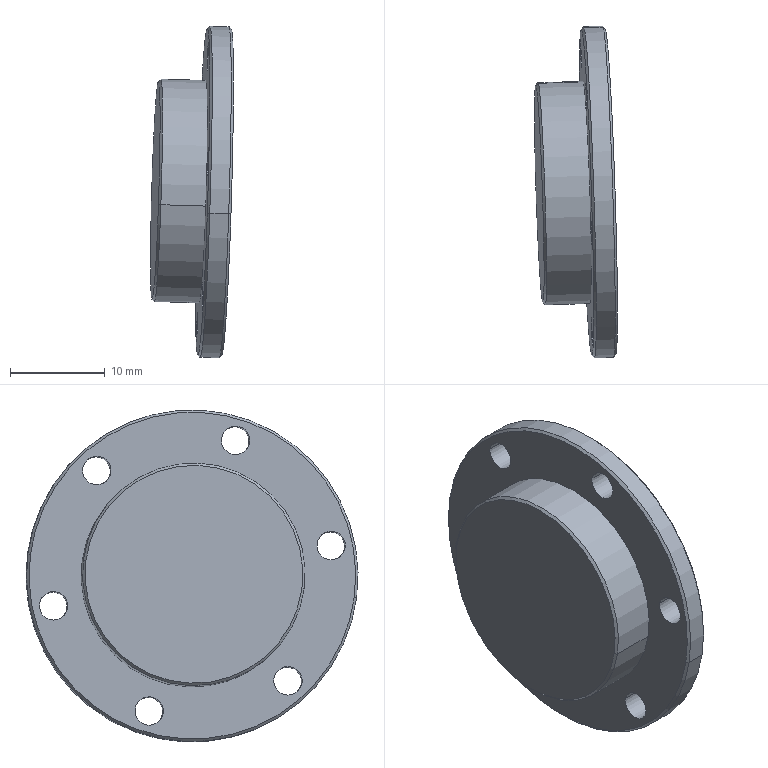Part | STEP file | 2026.6.15-Main Assembly图.sldasm-Part-114 | 1 solid | 30 faces | box 8.754 x 35.047 x 35.043 mm | volume 2415 mm3 | cylinder 18 | cone 8 | plane 4 | commonest cylinder face diameters 3 x12 20 x2 23.5 x2 35 x2
STEP:
#1=CARTESIAN_POINT('',(-1578.328,1431.126,3695.117));
#2=VERTEX_POINT('',#1);
#3=CARTESIAN_POINT('',(-1577.667,1408.329,3692.14));
#4=VERTEX_POINT('',#3);
#5=CARTESIAN_POINT('',(-1577.997,1419.728,3693.629));
#6=DIRECTION('',(-0.999,-0.03277,0.02917));
#7=DIRECTION('',(-0.02873,0.9912,0.1295));
#8=AXIS2_PLACEMENT_3D('',#5,#6,#7);
#9=CIRCLE('',#8,11.5);
#10=EDGE_CURVE('',#2,#4,#9,.T.);
#11=ORIENTED_EDGE('',*,*,#10,.F.);
#12=CARTESIAN_POINT('',(-1578.085,1431.382,3695.143));
#13=VERTEX_POINT('',#12);
#14=CARTESIAN_POINT('',(-1578.328,1431.126,3695.117));
#15=DIRECTION('',(0.6861,0.724,0.07092));
#16=VECTOR('',#15,1000.);
#17=LINE('',#14,#16);
#18=EDGE_CURVE('',#2,#13,#17,.T.);
#19=ORIENTED_EDGE('',*,*,#18,.T.);
#20=CARTESIAN_POINT('',(-1577.41,1408.09,3692.1));
#21=VERTEX_POINT('',#20);
#22=CARTESIAN_POINT('',(-1577.747,1419.736,3693.621));
#23=DIRECTION('',(0.999,0.03277,-0.02917));
#24=DIRECTION('',(-0.02873,0.9912,0.1295));
#25=AXIS2_PLACEMENT_3D('',#22,#23,#24);
#26=CIRCLE('',#25,11.75);
#27=EDGE_CURVE('',#21,#13,#26,.T.);
#28=ORIENTED_EDGE('',*,*,#27,.F.);
#29=CARTESIAN_POINT('',(-1577.667,1408.329,3692.14));
#30=DIRECTION('',(0.7267,-0.6777,-0.1122));
#31=VECTOR('',#30,1000.);
#32=LINE('',#29,#31);
#33=EDGE_CURVE('',#4,#21,#32,.T.);
#34=ORIENTED_EDGE('',*,*,#33,.F.);
#35=EDGE_LOOP('',(#11,#19,#28,#34));
#36=FACE_OUTER_BOUND('',#35,.T.);
#37=CARTESIAN_POINT('',(-1577.997,1419.728,3693.629));
#38=DIRECTION('',(0.999,0.03277,-0.02917));
#39=DIRECTION('',(0.02873,-0.9912,-0.1295));
#40=AXIS2_PLACEMENT_3D('',#37,#38,#39);
#41=CONICAL_SURFACE('',#40,11.5,0.7854);
#42=ADVANCED_FACE('',(#36),#41,.T.);
#43=CARTESIAN_POINT('',(-1573.498,1436.989,3695.716));
#44=VERTEX_POINT('',#43);
#45=CARTESIAN_POINT('',(-1572.506,1402.794,3691.249));
#46=VERTEX_POINT('',#45);
#47=CARTESIAN_POINT('',(-1573.002,1419.891,3693.483));
#48=DIRECTION('',(-0.999,-0.03277,0.02917));
#49=DIRECTION('',(-0.02873,0.9912,0.1295));
#50=AXIS2_PLACEMENT_3D('',#47,#48,#49);
#51=CIRCLE('',#50,17.25);
#52=EDGE_CURVE('',#44,#46,#51,.T.);
#53=ORIENTED_EDGE('',*,*,#52,.F.);
#54=CARTESIAN_POINT('',(-1573.255,1437.245,3695.741));
#55=VERTEX_POINT('',#54);
#56=CARTESIAN_POINT('',(-1573.498,1436.989,3695.716));
#57=DIRECTION('',(0.6861,0.724,0.07092));
#58=VECTOR('',#57,1000.);
#59=LINE('',#56,#58);
#60=EDGE_CURVE('',#44,#55,#59,.T.);
#61=ORIENTED_EDGE('',*,*,#60,.T.);
#62=CARTESIAN_POINT('',(-1572.249,1402.554,3691.21));
#63=VERTEX_POINT('',#62);
#64=CARTESIAN_POINT('',(-1572.752,1419.9,3693.475));
#65=DIRECTION('',(0.999,0.03277,-0.02917));
#66=DIRECTION('',(-0.02873,0.9912,0.1295));
#67=AXIS2_PLACEMENT_3D('',#64,#65,#66);
#68=CIRCLE('',#67,17.5);
#69=EDGE_CURVE('',#63,#55,#68,.T.);
#70=ORIENTED_EDGE('',*,*,#69,.F.);
#71=CARTESIAN_POINT('',(-1572.506,1402.794,3691.249));
#72=DIRECTION('',(0.7267,-0.6777,-0.1122));
#73=VECTOR('',#72,1000.);
#74=LINE('',#71,#73);
#75=EDGE_CURVE('',#46,#63,#74,.T.);
#76=ORIENTED_EDGE('',*,*,#75,.F.);
#77=EDGE_LOOP('',(#53,#61,#70,#76));
#78=FACE_OUTER_BOUND('',#77,.T.);
#79=CARTESIAN_POINT('',(-1573.002,1419.891,3693.483));
#80=DIRECTION('',(0.999,0.03277,-0.02917));
#81=DIRECTION('',(0.02873,-0.9912,-0.1295));
#82=AXIS2_PLACEMENT_3D('',#79,#80,#81);
#83=CONICAL_SURFACE('',#82,17.25,0.7854);
#84=ADVANCED_FACE('',(#78),#83,.T.);
#85=CARTESIAN_POINT('',(-1570.009,1402.876,3691.176));
#86=VERTEX_POINT('',#85);
#87=CARTESIAN_POINT('',(-1571.,1437.071,3695.643));
#88=VERTEX_POINT('',#87);
#89=CARTESIAN_POINT('',(-1570.504,1419.973,3693.41));
#90=DIRECTION('',(0.999,0.03277,-0.02917));
#91=DIRECTION('',(-0.02873,0.9912,0.1295));
#92=AXIS2_PLACEMENT_3D('',#89,#90,#91);
#93=CIRCLE('',#92,17.25);
#94=EDGE_CURVE('',#86,#88,#93,.T.);
#95=ORIENTED_EDGE('',*,*,#94,.F.);
#96=CARTESIAN_POINT('',(-1570.251,1402.62,3691.151));
#97=VERTEX_POINT('',#96);
#98=CARTESIAN_POINT('',(-1570.251,1402.62,3691.151));
#99=DIRECTION('',(-0.6861,-0.724,-0.07092));
#100=VECTOR('',#99,1000.);
#101=LINE('',#98,#100);
#102=EDGE_CURVE('',#86,#97,#101,.T.);
#103=ORIENTED_EDGE('',*,*,#102,.T.);
#104=CARTESIAN_POINT('',(-1571.257,1437.311,3695.683));
#105=VERTEX_POINT('',#104);
#106=CARTESIAN_POINT('',(-1570.754,1419.965,3693.417));
#107=DIRECTION('',(-0.999,-0.03277,0.02917));
#108=DIRECTION('',(-0.02873,0.9912,0.1295));
#109=AXIS2_PLACEMENT_3D('',#106,#107,#108);
#110=CIRCLE('',#109,17.5);
#111=EDGE_CURVE('',#105,#97,#110,.T.);
#112=ORIENTED_EDGE('',*,*,#111,.F.);
#113=CARTESIAN_POINT('',(-1571.257,1437.311,3695.683));
#114=DIRECTION('',(-0.7267,0.6777,0.1122));
#115=VECTOR('',#114,1000.);
#116=LINE('',#113,#115);
#117=EDGE_CURVE('',#88,#105,#116,.T.);
#118=ORIENTED_EDGE('',*,*,#117,.F.);
#119=EDGE_LOOP('',(#95,#103,#112,#118));
#120=FACE_OUTER_BOUND('',#119,.T.);
#121=CARTESIAN_POINT('',(-1570.754,1419.965,3693.417));
#122=DIRECTION('',(-0.999,-0.03277,0.02917));
#123=DIRECTION('',(-0.02873,0.9912,0.1295));
#124=AXIS2_PLACEMENT_3D('',#121,#122,#123);
#125=CONICAL_SURFACE('',#124,17.5,0.7854);
#126=ADVANCED_FACE('',(#120),#125,.T.);
#127=CARTESIAN_POINT('',(-1571.041,1429.877,3694.712));
#128=VERTEX_POINT('',#127);
#129=CARTESIAN_POINT('',(-1570.467,1410.053,3692.122));
#130=VERTEX_POINT('',#129);
#131=CARTESIAN_POINT('',(-1570.754,1419.965,3693.417));
#132=DIRECTION('',(0.999,0.03277,-0.02917));
#133=DIRECTION('',(-0.02873,0.9912,0.1295));
#134=AXIS2_PLACEMENT_3D('',#131,#132,#133);
#135=CIRCLE('',#134,10.);
#136=EDGE_CURVE('',#128,#130,#135,.T.);
#137=ORIENTED_EDGE('',*,*,#136,.F.);
#138=CARTESIAN_POINT('',(-1570.799,1430.133,3694.737));
#139=VERTEX_POINT('',#138);
#140=CARTESIAN_POINT('',(-1570.799,1430.133,3694.737));
#141=DIRECTION('',(0.6861,0.724,0.07092));
#142=VECTOR('',#141,1000.);
#143=LINE('',#140,#142);
#144=EDGE_CURVE('',#128,#139,#143,.T.);
#145=ORIENTED_EDGE('',*,*,#144,.T.);
#146=CARTESIAN_POINT('',(-1570.21,1409.814,3692.083));
#147=VERTEX_POINT('',#146);
#148=CARTESIAN_POINT('',(-1570.504,1419.973,3693.41));
#149=DIRECTION('',(-0.999,-0.03277,0.02917));
#150=DIRECTION('',(-0.02873,0.9912,0.1295));
#151=AXIS2_PLACEMENT_3D('',#148,#149,#150);
#152=CIRCLE('',#151,10.25);
#153=EDGE_CURVE('',#147,#139,#152,.T.);
#154=ORIENTED_EDGE('',*,*,#153,.F.);
#155=CARTESIAN_POINT('',(-1570.21,1409.814,3692.083));
#156=DIRECTION('',(0.7267,-0.6777,-0.1122));
#157=VECTOR('',#156,1000.);
#158=LINE('',#155,#157);
#159=EDGE_CURVE('',#130,#147,#158,.T.);
#160=ORIENTED_EDGE('',*,*,#159,.F.);
#161=EDGE_LOOP('',(#137,#145,#154,#160));
#162=FACE_OUTER_BOUND('',#161,.T.);
#163=CARTESIAN_POINT('',(-1570.504,1419.973,3693.41));
#164=DIRECTION('',(0.999,0.03277,-0.02917));
#165=DIRECTION('',(0.02873,-0.9912,-0.1295));
#166=AXIS2_PLACEMENT_3D('',#163,#164,#165);
#167=CONICAL_SURFACE('',#166,10.25,0.7854);
#168=ADVANCED_FACE('',(#162),#167,.F.);
#169=ORIENTED_EDGE('',*,*,#136,.T.);
#170=CARTESIAN_POINT('',(-1576.711,1409.849,3692.305));
#171=VERTEX_POINT('',#170);
#172=CARTESIAN_POINT('',(-1569.718,1410.078,3692.1));
#173=DIRECTION('',(-0.999,-0.03277,0.02917));
#174=VECTOR('',#173,1000.);
#175=LINE('',#172,#174);
#176=EDGE_CURVE('',#130,#171,#175,.T.);
#177=ORIENTED_EDGE('',*,*,#176,.T.);
#178=CARTESIAN_POINT('',(-1577.285,1429.672,3694.894));
#179=VERTEX_POINT('',#178);
#180=CARTESIAN_POINT('',(-1576.998,1419.76,3693.599));
#181=DIRECTION('',(0.999,0.03277,-0.02917));
#182=DIRECTION('',(-0.04387,0.7391,-0.6721));
#183=AXIS2_PLACEMENT_3D('',#180,#181,#182);
#184=CIRCLE('',#183,10.);
#185=EDGE_CURVE('',#179,#171,#184,.T.);
#186=ORIENTED_EDGE('',*,*,#185,.F.);
#187=CARTESIAN_POINT('',(-1570.292,1429.901,3694.69));
#188=DIRECTION('',(-0.999,-0.03277,0.02917));
#189=VECTOR('',#188,1000.);
#190=LINE('',#187,#189);
#191=EDGE_CURVE('',#128,#179,#190,.T.);
#192=ORIENTED_EDGE('',*,*,#191,.F.);
#193=EDGE_LOOP('',(#169,#177,#186,#192));
#194=FACE_OUTER_BOUND('',#193,.T.);
#195=CARTESIAN_POINT('',(-1570.005,1419.99,3693.395));
#196=DIRECTION('',(-0.999,-0.03277,0.02917));
#197=DIRECTION('',(-0.02873,0.9912,0.1295));
#198=AXIS2_PLACEMENT_3D('',#195,#196,#197);
#199=CYLINDRICAL_SURFACE('',#198,10.);
#200=ADVANCED_FACE('',(#194),#199,.F.);
#201=CARTESIAN_POINT('',(-1571.035,1433.134,3690.033));
#202=VERTEX_POINT('',#201);
#203=CARTESIAN_POINT('',(-1571.121,1436.107,3690.422));
#204=VERTEX_POINT('',#203);
#205=CARTESIAN_POINT('',(-1571.078,1434.621,3690.227));
#206=DIRECTION('',(-0.999,-0.03277,0.02917));
#207=DIRECTION('',(-0.04387,0.7391,-0.6721));
#208=AXIS2_PLACEMENT_3D('',#205,#206,#207);
#209=CIRCLE('',#208,1.5);
#210=EDGE_CURVE('',#202,#204,#209,.T.);
#211=ORIENTED_EDGE('',*,*,#210,.F.);
#212=CARTESIAN_POINT('',(-1573.532,1433.052,3690.106));
#213=VERTEX_POINT('',#212);
#214=CARTESIAN_POINT('',(-1571.035,1433.134,3690.033));
#215=DIRECTION('',(-0.999,-0.03277,0.02917));
#216=VECTOR('',#215,1000.);
#217=LINE('',#214,#216);
#218=EDGE_CURVE('',#202,#213,#217,.T.);
#219=ORIENTED_EDGE('',*,*,#218,.T.);
#220=CARTESIAN_POINT('',(-1573.618,1436.025,3690.495));
#221=VERTEX_POINT('',#220);
#222=CARTESIAN_POINT('',(-1573.575,1434.539,3690.3));
#223=DIRECTION('',(-0.999,-0.03277,0.02917));
#224=DIRECTION('',(-0.04387,0.7391,-0.6721));
#225=AXIS2_PLACEMENT_3D('',#222,#223,#224);
#226=CIRCLE('',#225,1.5);
#227=EDGE_CURVE('',#213,#221,#226,.T.);
#228=ORIENTED_EDGE('',*,*,#227,.T.);
#229=CARTESIAN_POINT('',(-1571.121,1436.107,3690.422));
#230=DIRECTION('',(-0.999,-0.03277,0.02917));
#231=VECTOR('',#230,1000.);
#232=LINE('',#229,#231);
#233=EDGE_CURVE('',#204,#221,#232,.T.);
#234=ORIENTED_EDGE('',*,*,#233,.F.);
#235=EDGE_LOOP('',(#211,#219,#228,#234));
#236=FACE_OUTER_BOUND('',#235,.T.);
#237=CARTESIAN_POINT('',(-1571.078,1434.621,3690.227));
#238=DIRECTION('',(-0.999,-0.03277,0.02917));
#239=DIRECTION('',(-0.02873,0.9912,0.1295));
#240=AXIS2_PLACEMENT_3D('',#237,#238,#239);
#241=CYLINDRICAL_SURFACE('',#240,1.5);
#242=ADVANCED_FACE('',(#236),#241,.F.);
#243=ORIENTED_EDGE('',*,*,#111,.T.);
#244=CARTESIAN_POINT('',(-1570.002,1402.628,3691.144));
#245=DIRECTION('',(-0.999,-0.03277,0.02917));
#246=VECTOR('',#245,1000.);
#247=LINE('',#244,#246);
#248=EDGE_CURVE('',#97,#63,#247,.T.);
#249=ORIENTED_EDGE('',*,*,#248,.T.);
#250=ORIENTED_EDGE('',*,*,#69,.T.);
#251=CARTESIAN_POINT('',(-1571.007,1437.319,3695.676));
#252=DIRECTION('',(-0.999,-0.03277,0.02917));
#253=VECTOR('',#252,1000.);
#254=LINE('',#251,#253);
#255=EDGE_CURVE('',#105,#55,#254,.T.);
#256=ORIENTED_EDGE('',*,*,#255,.F.);
#257=EDGE_LOOP('',(#243,#249,#250,#256));
#258=FACE_OUTER_BOUND('',#257,.T.);
#259=CARTESIAN_POINT('',(-1570.504,1419.973,3693.41));
#260=DIRECTION('',(-0.999,-0.03277,0.02917));
#261=DIRECTION('',(-0.02873,0.9912,0.1295));
#262=AXIS2_PLACEMENT_3D('',#259,#260,#261);
#263=CYLINDRICAL_SURFACE('',#262,17.5);
#264=ADVANCED_FACE('',(#258),#263,.T.);
#265=CARTESIAN_POINT('',(-1570.468,1428.578,3704.313));
#266=VERTEX_POINT('',#265);
#267=CARTESIAN_POINT('',(-1570.554,1431.551,3704.702));
#268=VERTEX_POINT('',#267);
#269=CARTESIAN_POINT('',(-1570.511,1430.065,3704.508));
#270=DIRECTION('',(-0.999,-0.03277,0.02917));
#271=DIRECTION('',(-0.04387,0.7391,-0.6721));
#272=AXIS2_PLACEMENT_3D('',#269,#270,#271);
#273=CIRCLE('',#272,1.5);
#274=EDGE_CURVE('',#266,#268,#273,.T.);
#275=ORIENTED_EDGE('',*,*,#274,.F.);
#276=CARTESIAN_POINT('',(-1572.966,1428.496,3704.386));
#277=VERTEX_POINT('',#276);
#278=CARTESIAN_POINT('',(-1570.468,1428.578,3704.313));
#279=DIRECTION('',(-0.999,-0.03277,0.02917));
#280=VECTOR('',#279,1000.);
#281=LINE('',#278,#280);
#282=EDGE_CURVE('',#266,#277,#281,.T.);
#283=ORIENTED_EDGE('',*,*,#282,.T.);
#284=CARTESIAN_POINT('',(-1573.052,1431.47,3704.775));
#285=VERTEX_POINT('',#284);
#286=CARTESIAN_POINT('',(-1573.009,1429.983,3704.581));
#287=DIRECTION('',(-0.999,-0.03277,0.02917));
#288=DIRECTION('',(-0.04387,0.7391,-0.6721));
#289=AXIS2_PLACEMENT_3D('',#286,#287,#288);
#290=CIRCLE('',#289,1.5);
#291=EDGE_CURVE('',#277,#285,#290,.T.);
#292=ORIENTED_EDGE('',*,*,#291,.T.);
#293=CARTESIAN_POINT('',(-1570.554,1431.551,3704.702));
#294=DIRECTION('',(-0.999,-0.03277,0.02917));
#295=VECTOR('',#294,1000.);
#296=LINE('',#293,#295);
#297=EDGE_CURVE('',#268,#285,#296,.T.);
#298=ORIENTED_EDGE('',*,*,#297,.F.);
#299=EDGE_LOOP('',(#275,#283,#292,#298));
#300=FACE_OUTER_BOUND('',#299,.T.);
#301=CARTESIAN_POINT('',(-1570.511,1430.065,3704.508));
#302=DIRECTION('',(-0.999,-0.03277,0.02917));
#303=DIRECTION('',(-0.02873,0.9912,0.1295));
#304=AXIS2_PLACEMENT_3D('',#301,#302,#303);
#305=CYLINDRICAL_SURFACE('',#304,1.5);
#306=ADVANCED_FACE('',(#300),#305,.F.);
#307=CARTESIAN_POINT('',(-1569.895,1413.931,3707.496));
#308=VERTEX_POINT('',#307);
#309=CARTESIAN_POINT('',(-1569.981,1416.904,3707.884));
#310=VERTEX_POINT('',#309);
#311=CARTESIAN_POINT('',(-1569.938,1415.417,3707.69));
#312=DIRECTION('',(-0.999,-0.03277,0.02917));
#313=DIRECTION('',(-0.04387,0.7391,-0.6721));
#314=AXIS2_PLACEMENT_3D('',#311,#312,#313);
#315=CIRCLE('',#314,1.5);
#316=EDGE_CURVE('',#308,#310,#315,.T.);
#317=ORIENTED_EDGE('',*,*,#316,.F.);
#318=CARTESIAN_POINT('',(-1572.392,1413.849,3707.569));
#319=VERTEX_POINT('',#318);
#320=CARTESIAN_POINT('',(-1569.895,1413.931,3707.496));
#321=DIRECTION('',(-0.999,-0.03277,0.02917));
#322=VECTOR('',#321,1000.);
#323=LINE('',#320,#322);
#324=EDGE_CURVE('',#308,#319,#323,.T.);
#325=ORIENTED_EDGE('',*,*,#324,.T.);
#326=CARTESIAN_POINT('',(-1572.479,1416.822,3707.957));
#327=VERTEX_POINT('',#326);
#328=CARTESIAN_POINT('',(-1572.436,1415.335,3707.763));
#329=DIRECTION('',(-0.999,-0.03277,0.02917));
#330=DIRECTION('',(-0.04387,0.7391,-0.6721));
#331=AXIS2_PLACEMENT_3D('',#328,#329,#330);
#332=CIRCLE('',#331,1.5);
#333=EDGE_CURVE('',#319,#327,#332,.T.);
#334=ORIENTED_EDGE('',*,*,#333,.T.);
#335=CARTESIAN_POINT('',(-1569.981,1416.904,3707.884));
#336=DIRECTION('',(-0.999,-0.03277,0.02917));
#337=VECTOR('',#336,1000.);
#338=LINE('',#335,#337);
#339=EDGE_CURVE('',#310,#327,#338,.T.);
#340=ORIENTED_EDGE('',*,*,#339,.F.);
#341=EDGE_LOOP('',(#317,#325,#334,#340));
#342=FACE_OUTER_BOUND('',#341,.T.);
#343=CARTESIAN_POINT('',(-1569.938,1415.417,3707.69));
#344=DIRECTION('',(-0.999,-0.03277,0.02917));
#345=DIRECTION('',(-0.02873,0.9912,0.1295));
#346=AXIS2_PLACEMENT_3D('',#343,#344,#345);
#347=CYLINDRICAL_SURFACE('',#346,1.5);
#348=ADVANCED_FACE('',(#342),#347,.F.);
#349=CARTESIAN_POINT('',(-1569.888,1403.839,3696.398));
#350=VERTEX_POINT('',#349);
#351=CARTESIAN_POINT('',(-1569.974,1406.813,3696.786));
#352=VERTEX_POINT('',#351);
#353=CARTESIAN_POINT('',(-1569.931,1405.326,3696.592));
#354=DIRECTION('',(-0.999,-0.03277,0.02917));
#355=DIRECTION('',(-0.04387,0.7391,-0.6721));
#356=AXIS2_PLACEMENT_3D('',#353,#354,#355);
#357=CIRCLE('',#356,1.5);
#358=EDGE_CURVE('',#350,#352,#357,.T.);
#359=ORIENTED_EDGE('',*,*,#358,.F.);
#360=CARTESIAN_POINT('',(-1572.386,1403.757,3696.471));
#361=VERTEX_POINT('',#360);
#362=CARTESIAN_POINT('',(-1569.888,1403.839,3696.398));
#363=DIRECTION('',(-0.999,-0.03277,0.02917));
#364=VECTOR('',#363,1000.);
#365=LINE('',#362,#364);
#366=EDGE_CURVE('',#350,#361,#365,.T.);
#367=ORIENTED_EDGE('',*,*,#366,.T.);
#368=CARTESIAN_POINT('',(-1572.472,1406.731,3696.859));
#369=VERTEX_POINT('',#368);
#370=CARTESIAN_POINT('',(-1572.429,1405.244,3696.665));
#371=DIRECTION('',(-0.999,-0.03277,0.02917));
#372=DIRECTION('',(-0.04387,0.7391,-0.6721));
#373=AXIS2_PLACEMENT_3D('',#370,#371,#372);
#374=CIRCLE('',#373,1.5);
#375=EDGE_CURVE('',#361,#369,#374,.T.);
#376=ORIENTED_EDGE('',*,*,#375,.T.);
#377=CARTESIAN_POINT('',(-1569.974,1406.813,3696.786));
#378=DIRECTION('',(-0.999,-0.03277,0.02917));
#379=VECTOR('',#378,1000.);
#380=LINE('',#377,#379);
#381=EDGE_CURVE('',#352,#369,#380,.T.);
#382=ORIENTED_EDGE('',*,*,#381,.F.);
#383=EDGE_LOOP('',(#359,#367,#376,#382));
#384=FACE_OUTER_BOUND('',#383,.T.);
#385=CARTESIAN_POINT('',(-1569.931,1405.326,3696.592));
#386=DIRECTION('',(-0.999,-0.03277,0.02917));
#387=DIRECTION('',(-0.02873,0.9912,0.1295));
#388=AXIS2_PLACEMENT_3D('',#385,#386,#387);
#389=CYLINDRICAL_SURFACE('',#388,1.5);
#390=ADVANCED_FACE('',(#384),#389,.F.);
#391=CARTESIAN_POINT('',(-1570.454,1408.395,3682.118));
#392=VERTEX_POINT('',#391);
#393=CARTESIAN_POINT('',(-1570.541,1411.369,3682.506));
#394=VERTEX_POINT('',#393);
#395=CARTESIAN_POINT('',(-1570.497,1409.882,3682.312));
#396=DIRECTION('',(-0.999,-0.03277,0.02917));
#397=DIRECTION('',(-0.04387,0.7391,-0.6721));
#398=AXIS2_PLACEMENT_3D('',#395,#396,#397);
#399=CIRCLE('',#398,1.5);
#400=EDGE_CURVE('',#392,#394,#399,.T.);
#401=ORIENTED_EDGE('',*,*,#400,.F.);
#402=CARTESIAN_POINT('',(-1572.952,1408.313,3682.191));
#403=VERTEX_POINT('',#402);
#404=CARTESIAN_POINT('',(-1570.454,1408.395,3682.118));
#405=DIRECTION('',(-0.999,-0.03277,0.02917));
#406=VECTOR('',#405,1000.);
#407=LINE('',#404,#406);
#408=EDGE_CURVE('',#392,#403,#407,.T.);
#409=ORIENTED_EDGE('',*,*,#408,.T.);
#410=CARTESIAN_POINT('',(-1573.038,1411.287,3682.579));
#411=VERTEX_POINT('',#410);
#412=CARTESIAN_POINT('',(-1572.995,1409.8,3682.385));
#413=DIRECTION('',(-0.999,-0.03277,0.02917));
#414=DIRECTION('',(-0.04387,0.7391,-0.6721));
#415=AXIS2_PLACEMENT_3D('',#412,#413,#414);
#416=CIRCLE('',#415,1.5);
#417=EDGE_CURVE('',#403,#411,#416,.T.);
#418=ORIENTED_EDGE('',*,*,#417,.T.);
#419=CARTESIAN_POINT('',(-1570.541,1411.369,3682.506));
#420=DIRECTION('',(-0.999,-0.03277,0.02917));
#421=VECTOR('',#420,1000.);
#422=LINE('',#419,#421);
#423=EDGE_CURVE('',#394,#411,#422,.T.);
#424=ORIENTED_EDGE('',*,*,#423,.F.);
#425=EDGE_LOOP('',(#401,#409,#418,#424));
#426=FACE_OUTER_BOUND('',#425,.T.);
#427=CARTESIAN_POINT('',(-1570.497,1409.882,3682.312));
#428=DIRECTION('',(-0.999,-0.03277,0.02917));
#429=DIRECTION('',(-0.02873,0.9912,0.1295));
#430=AXIS2_PLACEMENT_3D('',#427,#428,#429);
#431=CYLINDRICAL_SURFACE('',#430,1.5);
#432=ADVANCED_FACE('',(#426),#431,.F.);
#433=CARTESIAN_POINT('',(-1571.028,1423.043,3678.935));
#434=VERTEX_POINT('',#433);
#435=CARTESIAN_POINT('',(-1571.114,1426.016,3679.324));
#436=VERTEX_POINT('',#435);
#437=CARTESIAN_POINT('',(-1571.071,1424.529,3679.13));
#438=DIRECTION('',(-0.999,-0.03277,0.02917));
#439=DIRECTION('',(-0.04387,0.7391,-0.6721));
#440=AXIS2_PLACEMENT_3D('',#437,#438,#439);
#441=CIRCLE('',#440,1.5);
#442=EDGE_CURVE('',#434,#436,#441,.T.);
#443=ORIENTED_EDGE('',*,*,#442,.F.);
#444=CARTESIAN_POINT('',(-1573.525,1422.961,3679.008));
#445=VERTEX_POINT('',#444);
#446=CARTESIAN_POINT('',(-1571.028,1423.043,3678.935));
#447=DIRECTION('',(-0.999,-0.03277,0.02917));
#448=VECTOR('',#447,1000.);
#449=LINE('',#446,#448);
#450=EDGE_CURVE('',#434,#445,#449,.T.);
#451=ORIENTED_EDGE('',*,*,#450,.T.);
#452=CARTESIAN_POINT('',(-1573.612,1425.934,3679.397));
#453=VERTEX_POINT('',#452);
#454=CARTESIAN_POINT('',(-1573.568,1424.447,3679.202));
#455=DIRECTION('',(-0.999,-0.03277,0.02917));
#456=DIRECTION('',(-0.04387,0.7391,-0.6721));
#457=AXIS2_PLACEMENT_3D('',#454,#455,#456);
#458=CIRCLE('',#457,1.5);
#459=EDGE_CURVE('',#445,#453,#458,.T.);
#460=ORIENTED_EDGE('',*,*,#459,.T.);
#461=CARTESIAN_POINT('',(-1571.114,1426.016,3679.324));
#462=DIRECTION('',(-0.999,-0.03277,0.02917));
#463=VECTOR('',#462,1000.);
#464=LINE('',#461,#463);
#465=EDGE_CURVE('',#436,#453,#464,.T.);
#466=ORIENTED_EDGE('',*,*,#465,.F.);
#467=EDGE_LOOP('',(#443,#451,#460,#466));
#468=FACE_OUTER_BOUND('',#467,.T.);
#469=CARTESIAN_POINT('',(-1571.071,1424.529,3679.13));
#470=DIRECTION('',(-0.999,-0.03277,0.02917));
#471=DIRECTION('',(-0.02873,0.9912,0.1295));
#472=AXIS2_PLACEMENT_3D('',#469,#470,#471);
#473=CYLINDRICAL_SURFACE('',#472,1.5);
#474=ADVANCED_FACE('',(#468),#473,.F.);
#475=CARTESIAN_POINT('',(-1573.34,1431.538,3695.004));
#476=VERTEX_POINT('',#475);
#477=CARTESIAN_POINT('',(-1572.664,1408.245,3691.961));
#478=VERTEX_POINT('',#477);
#479=CARTESIAN_POINT('',(-1573.002,1419.891,3693.483));
#480=DIRECTION('',(-0.999,-0.03277,0.02917));
#481=DIRECTION('',(-0.04387,0.7391,-0.6721));
#482=AXIS2_PLACEMENT_3D('',#479,#480,#481);
#483=CIRCLE('',#482,11.75);
#484=EDGE_CURVE('',#476,#478,#483,.T.);
#485=ORIENTED_EDGE('',*,*,#484,.T.);
#486=CARTESIAN_POINT('',(-1572.664,1408.245,3691.961));
#487=DIRECTION('',(-0.999,-0.03277,0.02917));
#488=VECTOR('',#487,1000.);
#489=LINE('',#486,#488);
#490=EDGE_CURVE('',#478,#21,#489,.T.);
#491=ORIENTED_EDGE('',*,*,#490,.T.);
#492=ORIENTED_EDGE('',*,*,#27,.T.);
#493=CARTESIAN_POINT('',(-1573.34,1431.538,3695.004));
#494=DIRECTION('',(-0.999,-0.03277,0.02917));
#495=VECTOR('',#494,1000.);
#496=LINE('',#493,#495);
#497=EDGE_CURVE('',#476,#13,#496,.T.);
#498=ORIENTED_EDGE('',*,*,#497,.F.);
#499=EDGE_LOOP('',(#485,#491,#492,#498));
#500=FACE_OUTER_BOUND('',#499,.T.);
#501=CARTESIAN_POINT('',(-1573.002,1419.891,3693.483));
#502=DIRECTION('',(-0.999,-0.03277,0.02917));
#503=DIRECTION('',(-0.02873,0.9912,0.1295));
#504=AXIS2_PLACEMENT_3D('',#501,#502,#503);
#505=CYLINDRICAL_SURFACE('',#504,11.75);
#506=ADVANCED_FACE('',(#500),#505,.T.);
#507=ORIENTED_EDGE('',*,*,#490,.F.);
#508=CARTESIAN_POINT('',(-1573.002,1419.891,3693.483));
#509=DIRECTION('',(-0.999,-0.03277,0.02917));
#510=DIRECTION('',(-0.04387,0.7391,-0.6721));
#511=AXIS2_PLACEMENT_3D('',#508,#509,#510);
#512=CIRCLE('',#511,11.75);
#513=EDGE_CURVE('',#478,#476,#512,.T.);
#514=ORIENTED_EDGE('',*,*,#513,.T.);
#515=ORIENTED_EDGE('',*,*,#497,.T.);
#516=CARTESIAN_POINT('',(-1577.747,1419.736,3693.621));
#517=DIRECTION('',(0.999,0.03277,-0.02917));
#518=DIRECTION('',(-0.02873,0.9912,0.1295));
#519=AXIS2_PLACEMENT_3D('',#516,#517,#518);
#520=CIRCLE('',#519,11.75);
#521=EDGE_CURVE('',#13,#21,#520,.T.);
#522=ORIENTED_EDGE('',*,*,#521,.T.);
#523=EDGE_LOOP('',(#507,#514,#515,#522));
#524=FACE_OUTER_BOUND('',#523,.T.);
#525=CARTESIAN_POINT('',(-1573.002,1419.891,3693.483));
#526=DIRECTION('',(-0.999,-0.03277,0.02917));
#527=DIRECTION('',(-0.02873,0.9912,0.1295));
#528=AXIS2_PLACEMENT_3D('',#525,#526,#527);
#529=CYLINDRICAL_SURFACE('',#528,11.75);
#530=ADVANCED_FACE('',(#524),#529,.T.);
#531=CARTESIAN_POINT('',(-1577.997,1419.728,3693.629));
#532=DIRECTION('',(-0.999,-0.03277,0.02917));
#533=DIRECTION('',(-0.02873,0.9912,0.1295));
#534=AXIS2_PLACEMENT_3D('',#531,#532,#533);
#535=CIRCLE('',#534,11.5);
#536=EDGE_CURVE('',#4,#2,#535,.T.);
#537=ORIENTED_EDGE('',*,*,#536,.T.);
#538=ORIENTED_EDGE('',*,*,#10,.T.);
#539=EDGE_LOOP('',(#537,#538));
#540=FACE_OUTER_BOUND('',#539,.T.);
#541=CARTESIAN_POINT('',(-1577.997,1419.728,3693.629));
#542=DIRECTION('',(-0.999,-0.03277,0.02917));
#543=DIRECTION('',(-0.02873,0.9912,0.1295));
#544=AXIS2_PLACEMENT_3D('',#541,#542,#543);
#545=PLANE('',#544);
#546=ADVANCED_FACE('',(#540),#545,.T.);
#547=ORIENTED_EDGE('',*,*,#450,.F.);
#548=CARTESIAN_POINT('',(-1571.071,1424.529,3679.13));
#549=DIRECTION('',(-0.999,-0.03277,0.02917));
#550=DIRECTION('',(-0.04387,0.7391,-0.6721));
#551=AXIS2_PLACEMENT_3D('',#548,#549,#550);
#552=CIRCLE('',#551,1.5);
#553=EDGE_CURVE('',#436,#434,#552,.T.);
#554=ORIENTED_EDGE('',*,*,#553,.F.);
#555=ORIENTED_EDGE('',*,*,#465,.T.);
#556=CARTESIAN_POINT('',(-1573.568,1424.447,3679.202));
#557=DIRECTION('',(-0.999,-0.03277,0.02917));
#558=DIRECTION('',(-0.04387,0.7391,-0.6721));
#559=AXIS2_PLACEMENT_3D('',#556,#557,#558);
#560=CIRCLE('',#559,1.5);
#561=EDGE_CURVE('',#453,#445,#560,.T.);
#562=ORIENTED_EDGE('',*,*,#561,.T.);
#563=EDGE_LOOP('',(#547,#554,#555,#562));
#564=FACE_OUTER_BOUND('',#563,.T.);
#565=CARTESIAN_POINT('',(-1571.071,1424.529,3679.13));
#566=DIRECTION('',(-0.999,-0.03277,0.02917));
#567=DIRECTION('',(-0.02873,0.9912,0.1295));
#568=AXIS2_PLACEMENT_3D('',#565,#566,#567);
#569=CYLINDRICAL_SURFACE('',#568,1.5);
#570=ADVANCED_FACE('',(#564),#569,.F.);
#571=ORIENTED_EDGE('',*,*,#408,.F.);
#572=CARTESIAN_POINT('',(-1570.497,1409.882,3682.312));
#573=DIRECTION('',(-0.999,-0.03277,0.02917));
#574=DIRECTION('',(-0.04387,0.7391,-0.6721));
#575=AXIS2_PLACEMENT_3D('',#572,#573,#574);
#576=CIRCLE('',#575,1.5);
#577=EDGE_CURVE('',#394,#392,#576,.T.);
#578=ORIENTED_EDGE('',*,*,#577,.F.);
#579=ORIENTED_EDGE('',*,*,#423,.T.);
#580=CARTESIAN_POINT('',(-1572.995,1409.8,3682.385));
#581=DIRECTION('',(-0.999,-0.03277,0.02917));
#582=DIRECTION('',(-0.04387,0.7391,-0.6721));
#583=AXIS2_PLACEMENT_3D('',#580,#581,#582);
#584=CIRCLE('',#583,1.5);
#585=EDGE_CURVE('',#411,#403,#584,.T.);
#586=ORIENTED_EDGE('',*,*,#585,.T.);
#587=EDGE_LOOP('',(#571,#578,#579,#586));
#588=FACE_OUTER_BOUND('',#587,.T.);
#589=CARTESIAN_POINT('',(-1570.497,1409.882,3682.312));
#590=DIRECTION('',(-0.999,-0.03277,0.02917));
#591=DIRECTION('',(-0.02873,0.9912,0.1295));
#592=AXIS2_PLACEMENT_3D('',#589,#590,#591);
#593=CYLINDRICAL_SURFACE('',#592,1.5);
#594=ADVANCED_FACE('',(#588),#593,.F.);
#595=ORIENTED_EDGE('',*,*,#366,.F.);
#596=CARTESIAN_POINT('',(-1569.931,1405.326,3696.592));
#597=DIRECTION('',(-0.999,-0.03277,0.02917));
#598=DIRECTION('',(-0.04387,0.7391,-0.6721));
#599=AXIS2_PLACEMENT_3D('',#596,#597,#598);
#600=CIRCLE('',#599,1.5);
#601=EDGE_CURVE('',#352,#350,#600,.T.);
#602=ORIENTED_EDGE('',*,*,#601,.F.);
#603=ORIENTED_EDGE('',*,*,#381,.T.);
#604=CARTESIAN_POINT('',(-1572.429,1405.244,3696.665));
#605=DIRECTION('',(-0.999,-0.03277,0.02917));
#606=DIRECTION('',(-0.04387,0.7391,-0.6721));
#607=AXIS2_PLACEMENT_3D('',#604,#605,#606);
#608=CIRCLE('',#607,1.5);
#609=EDGE_CURVE('',#369,#361,#608,.T.);
#610=ORIENTED_EDGE('',*,*,#609,.T.);
#611=EDGE_LOOP('',(#595,#602,#603,#610));
#612=FACE_OUTER_BOUND('',#611,.T.);
#613=CARTESIAN_POINT('',(-1569.931,1405.326,3696.592));
#614=DIRECTION('',(-0.999,-0.03277,0.02917));
#615=DIRECTION('',(-0.02873,0.9912,0.1295));
#616=AXIS2_PLACEMENT_3D('',#613,#614,#615);
#617=CYLINDRICAL_SURFACE('',#616,1.5);
#618=ADVANCED_FACE('',(#612),#617,.F.);
#619=ORIENTED_EDGE('',*,*,#324,.F.);
#620=CARTESIAN_POINT('',(-1569.938,1415.417,3707.69));
#621=DIRECTION('',(-0.999,-0.03277,0.02917));
#622=DIRECTION('',(-0.04387,0.7391,-0.6721));
#623=AXIS2_PLACEMENT_3D('',#620,#621,#622);
#624=CIRCLE('',#623,1.5);
#625=EDGE_CURVE('',#310,#308,#624,.T.);
#626=ORIENTED_EDGE('',*,*,#625,.F.);
#627=ORIENTED_EDGE('',*,*,#339,.T.);
#628=CARTESIAN_POINT('',(-1572.436,1415.335,3707.763));
#629=DIRECTION('',(-0.999,-0.03277,0.02917));
#630=DIRECTION('',(-0.04387,0.7391,-0.6721));
#631=AXIS2_PLACEMENT_3D('',#628,#629,#630);
#632=CIRCLE('',#631,1.5);
#633=EDGE_CURVE('',#327,#319,#632,.T.);
#634=ORIENTED_EDGE('',*,*,#633,.T.);
#635=EDGE_LOOP('',(#619,#626,#627,#634));
#636=FACE_OUTER_BOUND('',#635,.T.);
#637=CARTESIAN_POINT('',(-1569.938,1415.417,3707.69));
#638=DIRECTION('',(-0.999,-0.03277,0.02917));
#639=DIRECTION('',(-0.02873,0.9912,0.1295));
#640=AXIS2_PLACEMENT_3D('',#637,#638,#639);
#641=CYLINDRICAL_SURFACE('',#640,1.5);
#642=ADVANCED_FACE('',(#636),#641,.F.);
#643=ORIENTED_EDGE('',*,*,#282,.F.);
#644=CARTESIAN_POINT('',(-1570.511,1430.065,3704.508));
#645=DIRECTION('',(-0.999,-0.03277,0.02917));
#646=DIRECTION('',(-0.04387,0.7391,-0.6721));
#647=AXIS2_PLACEMENT_3D('',#644,#645,#646);
#648=CIRCLE('',#647,1.5);
#649=EDGE_CURVE('',#268,#266,#648,.T.);
#650=ORIENTED_EDGE('',*,*,#649,.F.);
#651=ORIENTED_EDGE('',*,*,#297,.T.);
#652=CARTESIAN_POINT('',(-1573.009,1429.983,3704.581));
#653=DIRECTION('',(-0.999,-0.03277,0.02917));
#654=DIRECTION('',(-0.04387,0.7391,-0.6721));
#655=AXIS2_PLACEMENT_3D('',#652,#653,#654);
#656=CIRCLE('',#655,1.5);
#657=EDGE_CURVE('',#285,#277,#656,.T.);
#658=ORIENTED_EDGE('',*,*,#657,.T.);
#659=EDGE_LOOP('',(#643,#650,#651,#658));
#660=FACE_OUTER_BOUND('',#659,.T.);
#661=CARTESIAN_POINT('',(-1570.511,1430.065,3704.508));
#662=DIRECTION('',(-0.999,-0.03277,0.02917));
#663=DIRECTION('',(-0.02873,0.9912,0.1295));
#664=AXIS2_PLACEMENT_3D('',#661,#662,#663);
#665=CYLINDRICAL_SURFACE('',#664,1.5);
#666=ADVANCED_FACE('',(#660),#665,.F.);
#667=ORIENTED_EDGE('',*,*,#248,.F.);
#668=CARTESIAN_POINT('',(-1570.754,1419.965,3693.417));
#669=DIRECTION('',(-0.999,-0.03277,0.02917));
#670=DIRECTION('',(-0.02873,0.9912,0.1295));
#671=AXIS2_PLACEMENT_3D('',#668,#669,#670);
#672=CIRCLE('',#671,17.5);
#673=EDGE_CURVE('',#97,#105,#672,.T.);
#674=ORIENTED_EDGE('',*,*,#673,.T.);
#675=ORIENTED_EDGE('',*,*,#255,.T.);
#676=CARTESIAN_POINT('',(-1572.752,1419.9,3693.475));
#677=DIRECTION('',(0.999,0.03277,-0.02917));
#678=DIRECTION('',(-0.02873,0.9912,0.1295));
#679=AXIS2_PLACEMENT_3D('',#676,#677,#678);
#680=CIRCLE('',#679,17.5);
#681=EDGE_CURVE('',#55,#63,#680,.T.);
#682=ORIENTED_EDGE('',*,*,#681,.T.);
#683=EDGE_LOOP('',(#667,#674,#675,#682));
#684=FACE_OUTER_BOUND('',#683,.T.);
#685=CARTESIAN_POINT('',(-1570.504,1419.973,3693.41));
#686=DIRECTION('',(-0.999,-0.03277,0.02917));
#687=DIRECTION('',(-0.02873,0.9912,0.1295));
#688=AXIS2_PLACEMENT_3D('',#685,#686,#687);
#689=CYLINDRICAL_SURFACE('',#688,17.5);
#690=ADVANCED_FACE('',(#684),#689,.T.);
#691=ORIENTED_EDGE('',*,*,#218,.F.);
#692=CARTESIAN_POINT('',(-1571.078,1434.621,3690.227));
#693=DIRECTION('',(-0.999,-0.03277,0.02917));
#694=DIRECTION('',(-0.04387,0.7391,-0.6721));
#695=AXIS2_PLACEMENT_3D('',#692,#693,#694);
#696=CIRCLE('',#695,1.5);
#697=EDGE_CURVE('',#204,#202,#696,.T.);
#698=ORIENTED_EDGE('',*,*,#697,.F.);
#699=ORIENTED_EDGE('',*,*,#233,.T.);
#700=CARTESIAN_POINT('',(-1573.575,1434.539,3690.3));
#701=DIRECTION('',(-0.999,-0.03277,0.02917));
#702=DIRECTION('',(-0.04387,0.7391,-0.6721));
#703=AXIS2_PLACEMENT_3D('',#700,#701,#702);
#704=CIRCLE('',#703,1.5);
#705=EDGE_CURVE('',#221,#213,#704,.T.);
#706=ORIENTED_EDGE('',*,*,#705,.T.);
#707=EDGE_LOOP('',(#691,#698,#699,#706));
#708=FACE_OUTER_BOUND('',#707,.T.);
#709=CARTESIAN_POINT('',(-1571.078,1434.621,3690.227));
#710=DIRECTION('',(-0.999,-0.03277,0.02917));
#711=DIRECTION('',(-0.02873,0.9912,0.1295));
#712=AXIS2_PLACEMENT_3D('',#709,#710,#711);
#713=CYLINDRICAL_SURFACE('',#712,1.5);
#714=ADVANCED_FACE('',(#708),#713,.F.);
#715=ORIENTED_EDGE('',*,*,#153,.T.);
#716=CARTESIAN_POINT('',(-1570.504,1419.973,3693.41));
#717=DIRECTION('',(-0.999,-0.03277,0.02917));
#718=DIRECTION('',(-0.02873,0.9912,0.1295));
#719=AXIS2_PLACEMENT_3D('',#716,#717,#718);
#720=CIRCLE('',#719,10.25);
#721=EDGE_CURVE('',#139,#147,#720,.T.);
#722=ORIENTED_EDGE('',*,*,#721,.T.);
#723=EDGE_LOOP('',(#715,#722));
#724=FACE_BOUND('',#723,.T.);
#725=CARTESIAN_POINT('',(-1570.504,1419.973,3693.41));
#726=DIRECTION('',(0.999,0.03277,-0.02917));
#727=DIRECTION('',(-0.02873,0.9912,0.1295));
#728=AXIS2_PLACEMENT_3D('',#725,#726,#727);
#729=CIRCLE('',#728,17.25);
#730=EDGE_CURVE('',#88,#86,#729,.T.);
#731=ORIENTED_EDGE('',*,*,#730,.T.);
#732=ORIENTED_EDGE('',*,*,#94,.T.);
#733=EDGE_LOOP('',(#731,#732));
#734=FACE_OUTER_BOUND('',#733,.T.);
#735=ORIENTED_EDGE('',*,*,#649,.T.);
#736=ORIENTED_EDGE('',*,*,#274,.T.);
#737=EDGE_LOOP('',(#735,#736));
#738=FACE_BOUND('',#737,.T.);
#739=ORIENTED_EDGE('',*,*,#625,.T.);
#740=ORIENTED_EDGE('',*,*,#316,.T.);
#741=EDGE_LOOP('',(#739,#740));
#742=FACE_BOUND('',#741,.T.);
#743=ORIENTED_EDGE('',*,*,#601,.T.);
#744=ORIENTED_EDGE('',*,*,#358,.T.);
#745=EDGE_LOOP('',(#743,#744));
#746=FACE_BOUND('',#745,.T.);
#747=ORIENTED_EDGE('',*,*,#577,.T.);
#748=ORIENTED_EDGE('',*,*,#400,.T.);
#749=EDGE_LOOP('',(#747,#748));
#750=FACE_BOUND('',#749,.T.);
#751=ORIENTED_EDGE('',*,*,#553,.T.);
#752=ORIENTED_EDGE('',*,*,#442,.T.);
#753=EDGE_LOOP('',(#751,#752));
#754=FACE_BOUND('',#753,.T.);
#755=ORIENTED_EDGE('',*,*,#697,.T.);
#756=ORIENTED_EDGE('',*,*,#210,.T.);
#757=EDGE_LOOP('',(#755,#756));
#758=FACE_BOUND('',#757,.T.);
#759=CARTESIAN_POINT('',(-1570.508,1425.019,3698.959));
#760=DIRECTION('',(-0.999,-0.03277,0.02917));
#761=DIRECTION('',(-0.02873,0.9912,0.1295));
#762=AXIS2_PLACEMENT_3D('',#759,#760,#761);
#763=PLANE('',#762);
#764=ADVANCED_FACE('',(#724,#734,#738,#742,#746,#750,#754,#758),#763,.F.);
#765=CARTESIAN_POINT('',(-1573.002,1419.891,3693.483));
#766=DIRECTION('',(-0.999,-0.03277,0.02917));
#767=DIRECTION('',(-0.02873,0.9912,0.1295));
#768=AXIS2_PLACEMENT_3D('',#765,#766,#767);
#769=CIRCLE('',#768,17.25);
#770=EDGE_CURVE('',#46,#44,#769,.T.);
#771=ORIENTED_EDGE('',*,*,#770,.T.);
#772=ORIENTED_EDGE('',*,*,#52,.T.);
#773=EDGE_LOOP('',(#771,#772));
#774=FACE_OUTER_BOUND('',#773,.T.);
#775=ORIENTED_EDGE('',*,*,#484,.F.);
#776=ORIENTED_EDGE('',*,*,#513,.F.);
#777=EDGE_LOOP('',(#775,#776));
#778=FACE_BOUND('',#777,.T.);
#779=ORIENTED_EDGE('',*,*,#657,.F.);
#780=ORIENTED_EDGE('',*,*,#291,.F.);
#781=EDGE_LOOP('',(#779,#780));
#782=FACE_BOUND('',#781,.T.);
#783=ORIENTED_EDGE('',*,*,#633,.F.);
#784=ORIENTED_EDGE('',*,*,#333,.F.);
#785=EDGE_LOOP('',(#783,#784));
#786=FACE_BOUND('',#785,.T.);
#787=ORIENTED_EDGE('',*,*,#609,.F.);
#788=ORIENTED_EDGE('',*,*,#375,.F.);
#789=EDGE_LOOP('',(#787,#788));
#790=FACE_BOUND('',#789,.T.);
#791=ORIENTED_EDGE('',*,*,#585,.F.);
#792=ORIENTED_EDGE('',*,*,#417,.F.);
#793=EDGE_LOOP('',(#791,#792));
#794=FACE_BOUND('',#793,.T.);
#795=ORIENTED_EDGE('',*,*,#561,.F.);
#796=ORIENTED_EDGE('',*,*,#459,.F.);
#797=EDGE_LOOP('',(#795,#796));
#798=FACE_BOUND('',#797,.T.);
#799=ORIENTED_EDGE('',*,*,#705,.F.);
#800=ORIENTED_EDGE('',*,*,#227,.F.);
#801=EDGE_LOOP('',(#799,#800));
#802=FACE_BOUND('',#801,.T.);
#803=CARTESIAN_POINT('',(-1573.005,1424.937,3699.032));
#804=DIRECTION('',(-0.999,-0.03277,0.02917));
#805=DIRECTION('',(-0.02873,0.9912,0.1295));
#806=AXIS2_PLACEMENT_3D('',#803,#804,#805);
#807=PLANE('',#806);
#808=ADVANCED_FACE('',(#774,#778,#782,#786,#790,#794,#798,#802),#807,.T.);
#809=ORIENTED_EDGE('',*,*,#176,.F.);
#810=CARTESIAN_POINT('',(-1570.754,1419.965,3693.417));
#811=DIRECTION('',(0.999,0.03277,-0.02917));
#812=DIRECTION('',(-0.02873,0.9912,0.1295));
#813=AXIS2_PLACEMENT_3D('',#810,#811,#812);
#814=CIRCLE('',#813,10.);
#815=EDGE_CURVE('',#130,#128,#814,.T.);
#816=ORIENTED_EDGE('',*,*,#815,.T.);
#817=ORIENTED_EDGE('',*,*,#191,.T.);
#818=CARTESIAN_POINT('',(-1576.998,1419.76,3693.599));
#819=DIRECTION('',(0.999,0.03277,-0.02917));
#820=DIRECTION('',(-0.04387,0.7391,-0.6721));
#821=AXIS2_PLACEMENT_3D('',#818,#819,#820);
#822=CIRCLE('',#821,10.);
#823=EDGE_CURVE('',#171,#179,#822,.T.);
#824=ORIENTED_EDGE('',*,*,#823,.F.);
#825=EDGE_LOOP('',(#809,#816,#817,#824));
#826=FACE_OUTER_BOUND('',#825,.T.);
#827=CARTESIAN_POINT('',(-1570.005,1419.99,3693.395));
#828=DIRECTION('',(-0.999,-0.03277,0.02917));
#829=DIRECTION('',(-0.02873,0.9912,0.1295));
#830=AXIS2_PLACEMENT_3D('',#827,#828,#829);
#831=CYLINDRICAL_SURFACE('',#830,10.);
#832=ADVANCED_FACE('',(#826),#831,.F.);
#833=ORIENTED_EDGE('',*,*,#185,.T.);
#834=ORIENTED_EDGE('',*,*,#823,.T.);
#835=EDGE_LOOP('',(#833,#834));
#836=FACE_OUTER_BOUND('',#835,.T.);
#837=CARTESIAN_POINT('',(-1576.998,1419.76,3693.599));
#838=DIRECTION('',(-0.999,-0.03277,0.02917));
#839=DIRECTION('',(-0.02873,0.9912,0.1295));
#840=AXIS2_PLACEMENT_3D('',#837,#838,#839);
#841=PLANE('',#840);
#842=ADVANCED_FACE('',(#836),#841,.F.);
#843=ORIENTED_EDGE('',*,*,#144,.F.);
#844=ORIENTED_EDGE('',*,*,#815,.F.);
#845=ORIENTED_EDGE('',*,*,#159,.T.);
#846=ORIENTED_EDGE('',*,*,#721,.F.);
#847=EDGE_LOOP('',(#843,#844,#845,#846));
#848=FACE_OUTER_BOUND('',#847,.T.);
#849=CARTESIAN_POINT('',(-1570.504,1419.973,3693.41));
#850=DIRECTION('',(0.999,0.03277,-0.02917));
#851=DIRECTION('',(0.02873,-0.9912,-0.1295));
#852=AXIS2_PLACEMENT_3D('',#849,#850,#851);
#853=CONICAL_SURFACE('',#852,10.25,0.7854);
#854=ADVANCED_FACE('',(#848),#853,.F.);
#855=ORIENTED_EDGE('',*,*,#102,.F.);
#856=ORIENTED_EDGE('',*,*,#730,.F.);
#857=ORIENTED_EDGE('',*,*,#117,.T.);
#858=ORIENTED_EDGE('',*,*,#673,.F.);
#859=EDGE_LOOP('',(#855,#856,#857,#858));
#860=FACE_OUTER_BOUND('',#859,.T.);
#861=CARTESIAN_POINT('',(-1570.754,1419.965,3693.417));
#862=DIRECTION('',(-0.999,-0.03277,0.02917));
#863=DIRECTION('',(-0.02873,0.9912,0.1295));
#864=AXIS2_PLACEMENT_3D('',#861,#862,#863);
#865=CONICAL_SURFACE('',#864,17.5,0.7854);
#866=ADVANCED_FACE('',(#860),#865,.T.);
#867=ORIENTED_EDGE('',*,*,#60,.F.);
#868=ORIENTED_EDGE('',*,*,#770,.F.);
#869=ORIENTED_EDGE('',*,*,#75,.T.);
#870=ORIENTED_EDGE('',*,*,#681,.F.);
#871=EDGE_LOOP('',(#867,#868,#869,#870));
#872=FACE_OUTER_BOUND('',#871,.T.);
#873=CARTESIAN_POINT('',(-1573.002,1419.891,3693.483));
#874=DIRECTION('',(0.999,0.03277,-0.02917));
#875=DIRECTION('',(0.02873,-0.9912,-0.1295));
#876=AXIS2_PLACEMENT_3D('',#873,#874,#875);
#877=CONICAL_SURFACE('',#876,17.25,0.7854);
#878=ADVANCED_FACE('',(#872),#877,.T.);
#879=ORIENTED_EDGE('',*,*,#18,.F.);
#880=ORIENTED_EDGE('',*,*,#536,.F.);
#881=ORIENTED_EDGE('',*,*,#33,.T.);
#882=ORIENTED_EDGE('',*,*,#521,.F.);
#883=EDGE_LOOP('',(#879,#880,#881,#882));
#884=FACE_OUTER_BOUND('',#883,.T.);
#885=CARTESIAN_POINT('',(-1577.997,1419.728,3693.629));
#886=DIRECTION('',(0.999,0.03277,-0.02917));
#887=DIRECTION('',(0.02873,-0.9912,-0.1295));
#888=AXIS2_PLACEMENT_3D('',#885,#886,#887);
#889=CONICAL_SURFACE('',#888,11.5,0.7854);
#890=ADVANCED_FACE('',(#884),#889,.T.);
#891=CLOSED_SHELL('',(#42,#84,#126,#168,#200,#242,#264,#306,#348,#390,#432,#474,#506,#530,#546,#570,#594,#618,#642,#666,#690,#714,#764,#808,#832,#842,#854,#866,#878,#890));
#892=MANIFOLD_SOLID_BREP('',#891);
#893=CARTESIAN_POINT('',(0.,0.,0.));
#894=DIRECTION('',(0.,0.,1.));
#895=DIRECTION('',(1.,0.,0.));
#896=AXIS2_PLACEMENT_3D('',#893,#894,#895);
#897=(LENGTH_UNIT()NAMED_UNIT(*)SI_UNIT(.MILLI.,.METRE.));
#898=UNCERTAINTY_MEASURE_WITH_UNIT(LENGTH_MEASURE(0.00001),#897,'','');
#899=(NAMED_UNIT(*)PLANE_ANGLE_UNIT()SI_UNIT($,.RADIAN.));
#900=(NAMED_UNIT(*)SI_UNIT($,.STERADIAN.)SOLID_ANGLE_UNIT());
#901=(GEOMETRIC_REPRESENTATION_CONTEXT(3)GLOBAL_UNCERTAINTY_ASSIGNED_CONTEXT((#898))GLOBAL_UNIT_ASSIGNED_CONTEXT((#897,#899,#900))REPRESENTATION_CONTEXT('',''));
#902=ADVANCED_BREP_SHAPE_REPRESENTATION('',(#892,#896),#901);